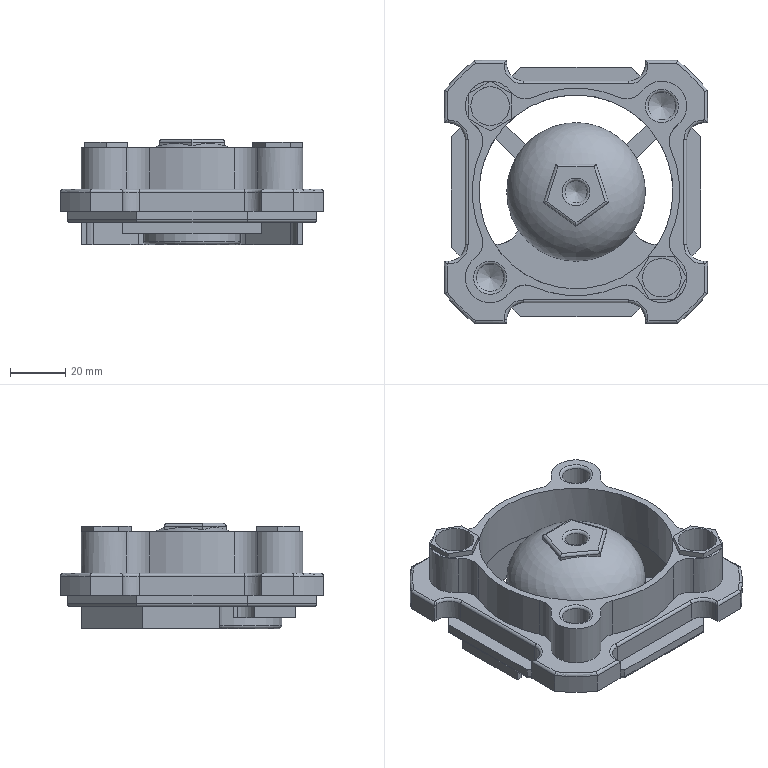NC program | NX | posted with a generic post | part box 95 x 95 x 38 mm
Lines 3621 to 4419 of 59038:
(FIXED_CONTOUR_2 , TOOL : D10R1)
N7186 M6
N7188 G54
N7190 G17 G0 G90 X-4.223 Y-29.7 S3000 M3
N7192 G43 Z10. H0
N7194 Z-8.
N7196 G94 G1 Z-19. F2500.
N7198 Y-29.698 Z-18.791
N7200 X-4.222 Y-29.695 Z-18.644
N7202 Y-29.691 Z-18.511
N7204 X-4.216 Y-29.652 Z-17.848
N7206 X-4.211 Y-29.614 Z-17.452
N7208 X-4.2 Y-29.537 Z-16.864
N7210 X-4.189 Y-29.461 Z-16.413
N7212 X-4.178 Y-29.384 Z-16.03
N7214 X-4.156 Y-29.231 Z-15.382
N7216 X-4.135 Y-29.078 Z-14.842
N7218 X-4.113 Y-28.925 Z-14.361
N7220 X-4.091 Y-28.772 Z-13.934
N7222 X-4.069 Y-28.619 Z-13.541
N7224 X-4.047 Y-28.466 Z-13.176
N7226 X-4.004 Y-28.16 Z-12.513
N7228 X-3.96 Y-27.853 Z-11.919
N7230 X-3.917 Y-27.547 Z-11.378
N7232 X-3.873 Y-27.241 Z-10.881
N7234 X-3.83 Y-26.935 Z-10.417
N7236 X-3.786 Y-26.629 Z-9.983
N7238 X-3.743 Y-26.322 Z-9.575
N7240 X-3.699 Y-26.016 Z-9.189
N7242 X-3.656 Y-25.71 Z-8.821
N7244 X-3.612 Y-25.404 Z-8.473
N7246 X-3.569 Y-25.098 Z-8.141
N7248 X-3.525 Y-24.791 Z-7.823
N7250 X-3.438 Y-24.179 Z-7.226
N7252 X-3.351 Y-23.567 Z-6.674
N7254 X-3.264 Y-22.954 Z-6.162
N7256 X-3.177 Y-22.342 Z-5.685
N7258 X-3.09 Y-21.73 Z-5.239
N7260 X-3.003 Y-21.117 Z-4.823
N7262 X-2.915 Y-20.505 Z-4.432
N7264 X-2.828 Y-19.892 Z-4.065
N7266 X-2.717 Y-19.109 Z-3.628
N7268 X-2.606 Y-18.325 Z-3.224
N7270 X-2.494 Y-17.541 Z-2.851
N7272 X-2.383 Y-16.757 Z-2.506
N7274 X-2.382 Y-16.756 Z-2.
N7276 Y-16.755 Z-1.929
N7278 X-2.381 Y-16.748 Z-1.827
N7280 X-2.38 Y-16.741 Z-1.766
N7282 X-2.378 Y-16.727 Z-1.683
N7284 X-2.374 Y-16.7 Z-1.551
N7286 X-2.367 Y-16.645 Z-1.371
N7288 X-2.359 Y-16.59 Z-1.237
N7290 X-2.351 Y-16.535 Z-1.128
N7292 X-2.335 Y-16.425 Z-0.946
N7294 X-2.32 Y-16.315 Z-0.8
N7296 X-2.304 Y-16.204 Z-0.676
N7298 X-2.288 Y-16.094 Z-0.571
N7300 X-2.257 Y-15.874 Z-0.4
N7302 X-2.226 Y-15.654 Z-0.269
N7304 X-2.194 Y-15.434 Z-0.168
N7306 X-2.163 Y-15.213 Z-0.093
N7308 X-2.132 Y-14.993 Z-0.041
N7310 X-2.11 Y-14.84 Z-0.019
N7312 X-2.088 Y-14.687 Z-0.005
N7314 X-2.045 Y-14.381 Z0.
N7316 X-1.434 Y-10.083
N7318 X-1.371 Y-10.128
N7320 X-1.953 Y-14.422
N7322 X-1.994 Y-14.728 Z-0.004
N7324 X-2.015 Y-14.881 Z-0.017
N7326 X-2.036 Y-15.034 Z-0.038
N7328 X-2.066 Y-15.256 Z-0.089
N7330 X-2.096 Y-15.478 Z-0.164
N7332 X-2.126 Y-15.7 Z-0.265
N7334 X-2.156 Y-15.922 Z-0.396
N7336 X-2.186 Y-16.144 Z-0.566
N7338 X-2.201 Y-16.255 Z-0.672
N7340 X-2.216 Y-16.366 Z-0.795
N7342 X-2.231 Y-16.478 Z-0.942
N7344 X-2.246 Y-16.589 Z-1.124
N7346 X-2.254 Y-16.644 Z-1.234
N7348 X-2.261 Y-16.7 Z-1.368
N7350 X-2.269 Y-16.755 Z-1.548
N7352 X-2.272 Y-16.783 Z-1.681
N7354 X-2.274 Y-16.797 Z-1.763
N7356 X-2.276 Y-16.811 Z-1.922
N7358 Y-16.812 Z-2.
N7360 Y-16.813 Z-2.523
N7362 X-2.382 Y-17.592 Z-2.867
N7364 X-2.487 Y-18.37 Z-3.238
N7366 X-2.593 Y-19.149 Z-3.64
N7368 X-2.698 Y-19.928 Z-4.075
N7370 X-2.781 Y-20.54 Z-4.443
N7372 X-2.864 Y-21.152 Z-4.833
N7374 X-2.947 Y-21.764 Z-5.249
N7376 X-3.03 Y-22.376 Z-5.695
N7378 X-3.112 Y-22.987 Z-6.172
N7380 X-3.195 Y-23.599 Z-6.684
N7382 X-3.278 Y-24.211 Z-7.235
N7384 X-3.361 Y-24.823 Z-7.832
N7386 X-3.402 Y-25.129 Z-8.15
N7388 X-3.444 Y-25.435 Z-8.482
N7390 X-3.485 Y-25.74 Z-8.83
N7392 X-3.527 Y-26.046 Z-9.197
N7394 X-3.568 Y-26.352 Z-9.583
N7396 X-3.609 Y-26.658 Z-9.99
N7398 X-3.651 Y-26.964 Z-10.424
N7400 X-3.692 Y-27.27 Z-10.887
N7402 X-3.734 Y-27.576 Z-11.385
N7404 X-3.775 Y-27.882 Z-11.924
N7406 X-3.816 Y-28.188 Z-12.518
N7408 X-3.858 Y-28.494 Z-13.181
N7410 X-3.879 Y-28.647 Z-13.545
N7412 X-3.899 Y-28.799 Z-13.938
N7414 X-3.92 Y-28.952 Z-14.365
N7416 X-3.941 Y-29.105 Z-14.845
N7418 X-3.961 Y-29.258 Z-15.385
N7420 X-3.982 Y-29.411 Z-16.031
N7422 X-3.992 Y-29.488 Z-16.414
N7424 X-4.003 Y-29.564 Z-16.864
N7426 X-4.013 Y-29.641 Z-17.451
N7428 X-4.018 Y-29.679 Z-17.846
N7430 X-4.024 Y-29.717 Z-18.505
N7432 X-4.025 Y-29.727 Z-19.
N7434 X-3.827 Y-29.754
N7436 X-3.826 Y-29.744 Z-18.499
N7438 X-3.821 Y-29.706 Z-17.845
N7440 X-3.816 Y-29.667 Z-17.45
N7442 X-3.806 Y-29.591 Z-16.865
N7444 X-3.796 Y-29.515 Z-16.415
N7446 X-3.786 Y-29.438 Z-16.033
N7448 X-3.767 Y-29.285 Z-15.387
N7450 X-3.747 Y-29.133 Z-14.848
N7452 X-3.727 Y-28.98 Z-14.369
N7454 X-3.708 Y-28.827 Z-13.942
N7456 X-3.688 Y-28.674 Z-13.549
N7458 X-3.668 Y-28.521 Z-13.185
N7460 X-3.629 Y-28.216 Z-12.524
N7462 X-3.59 Y-27.91 Z-11.93
N7464 X-3.55 Y-27.605 Z-11.391
N7466 X-3.511 Y-27.299 Z-10.894
N7468 X-3.472 Y-26.993 Z-10.431
N7470 X-3.432 Y-26.688 Z-9.998
N7472 X-3.393 Y-26.382 Z-9.591
N7474 X-3.354 Y-26.077 Z-9.205
N7476 X-3.315 Y-25.771 Z-8.839
N7478 X-3.275 Y-25.465 Z-8.49
N7480 X-3.236 Y-25.16 Z-8.159
N7482 X-3.197 Y-24.854 Z-7.841
N7484 X-3.118 Y-24.243 Z-7.245
N7486 X-3.039 Y-23.632 Z-6.694
N7488 X-2.961 Y-23.021 Z-6.182
N7490 X-2.882 Y-22.409 Z-5.705
N7492 X-2.804 Y-21.798 Z-5.26
N7494 X-2.725 Y-21.187 Z-4.844
N7496 X-2.646 Y-20.576 Z-4.453
N7498 X-2.568 Y-19.965 Z-4.086
N7500 X-2.468 Y-19.19 Z-3.653
N7502 X-2.368 Y-18.415 Z-3.252
N7504 X-2.269 Y-17.641 Z-2.882
N7506 X-2.169 Y-16.866 Z-2.539
N7508 Y-16.865 Z-2.
N7510 Y-16.864 Z-1.934
N7512 Y-16.861 Z-1.868
N7514 X-2.168 Y-16.857 Z-1.828
N7516 X-2.167 Y-16.85 Z-1.765
N7518 X-2.165 Y-16.836 Z-1.682
N7520 X-2.162 Y-16.808 Z-1.548
N7522 X-2.155 Y-16.752 Z-1.367
N7524 X-2.147 Y-16.696 Z-1.232
N7526 X-2.14 Y-16.64 Z-1.122
N7528 X-2.126 Y-16.529 Z-0.94
N7530 X-2.111 Y-16.417 Z-0.792
N7532 X-2.097 Y-16.305 Z-0.668
N7534 X-2.083 Y-16.193 Z-0.563
N7536 X-2.054 Y-15.97 Z-0.392
N7538 X-2.025 Y-15.746 Z-0.261
N7540 X-1.996 Y-15.522 Z-0.161
N7542 X-1.968 Y-15.299 Z-0.087
N7544 X-1.939 Y-15.075 Z-0.037
N7546 X-1.919 Y-14.922 Z-0.016
N7548 X-1.9 Y-14.769 Z-0.004
N7550 X-1.86 Y-14.464 Z0.
N7552 X-1.309 Y-10.174
N7554 X-1.245 Y-10.22
N7556 X-1.767 Y-14.505
N7558 X-1.805 Y-14.81 Z-0.004
N7560 X-1.823 Y-14.963 Z-0.015
N7562 X-1.842 Y-15.115 Z-0.035
N7564 X-1.869 Y-15.34 Z-0.085
N7566 X-1.897 Y-15.565 Z-0.158
N7568 X-1.924 Y-15.79 Z-0.259
N7570 X-1.951 Y-16.015 Z-0.389
N7572 X-1.979 Y-16.24 Z-0.56
N7574 X-1.992 Y-16.352 Z-0.665
N7576 X-2.006 Y-16.464 Z-0.789
N7578 X-2.02 Y-16.577 Z-0.937
N7580 X-2.034 Y-16.689 Z-1.119
N7582 X-2.04 Y-16.745 Z-1.23
N7584 X-2.047 Y-16.802 Z-1.365
N7586 X-2.054 Y-16.858 Z-1.545
N7588 X-2.058 Y-16.886 Z-1.678
N7590 X-2.059 Y-16.9 Z-1.761
N7592 X-2.061 Y-16.914 Z-1.918
N7594 Y-16.916 Z-2.
N7596 Z-2.554
N7598 X-2.155 Y-17.687 Z-2.896
N7600 X-2.249 Y-18.458 Z-3.265
N7602 X-2.343 Y-19.229 Z-3.665
N7604 X-2.437 Y-20. Z-4.096
N7606 X-2.511 Y-20.61 Z-4.464
N7608 X-2.586 Y-21.221 Z-4.854
N7610 X-2.66 Y-21.831 Z-5.27
N7612 X-2.734 Y-22.442 Z-5.715
N7614 X-2.809 Y-23.052 Z-6.192
N7616 X-2.883 Y-23.663 Z-6.703
N7618 X-2.958 Y-24.273 Z-7.254
N7620 X-3.032 Y-24.884 Z-7.85
N7622 X-3.069 Y-25.189 Z-8.167
N7624 X-3.106 Y-25.495 Z-8.498
N7626 X-3.144 Y-25.8 Z-8.846
N7628 X-3.181 Y-26.105 Z-9.212
N7630 X-3.218 Y-26.41 Z-9.598
N7632 X-3.255 Y-26.716 Z-10.004
N7634 X-3.292 Y-27.021 Z-10.437
N7636 X-3.33 Y-27.326 Z-10.899
N7638 X-3.367 Y-27.631 Z-11.396
N7640 X-3.404 Y-27.937 Z-11.934
N7642 X-3.441 Y-28.242 Z-12.527
N7644 X-3.478 Y-28.547 Z-13.188
N7646 X-3.497 Y-28.7 Z-13.551
N7648 X-3.516 Y-28.852 Z-13.943
N7650 X-3.534 Y-29.005 Z-14.369
N7652 X-3.553 Y-29.158 Z-14.847
N7654 X-3.571 Y-29.31 Z-15.385
N7656 X-3.59 Y-29.463 Z-16.029
N7658 X-3.599 Y-29.539 Z-16.41
N7660 X-3.609 Y-29.616 Z-16.857
N7662 X-3.618 Y-29.692 Z-17.44
N7664 X-3.623 Y-29.73 Z-17.83
N7666 X-3.627 Y-29.768 Z-18.462
N7668 X-3.628 Y-29.778 Z-19.
N7670 X-3.43 Y-29.802
N7672 X-3.429 Y-29.792 Z-18.504
N7674 X-3.424 Y-29.754 Z-17.848
N7676 X-3.42 Y-29.716 Z-17.455
N7678 X-3.411 Y-29.639 Z-16.87
N7680 X-3.402 Y-29.563 Z-16.421
N7682 X-3.394 Y-29.487 Z-16.039
N7684 X-3.376 Y-29.335 Z-15.394
N7686 X-3.359 Y-29.182 Z-14.856
N7688 X-3.341 Y-29.03 Z-14.378
N7690 X-3.324 Y-28.877 Z-13.951
N7692 X-3.306 Y-28.725 Z-13.56
N7694 X-3.288 Y-28.572 Z-13.196
N7696 X-3.253 Y-28.267 Z-12.536
N7698 X-3.218 Y-27.962 Z-11.943
N7700 X-3.183 Y-27.658 Z-11.406
N7702 X-3.148 Y-27.353 Z-10.909
N7704 X-3.113 Y-27.048 Z-10.447
N7706 X-3.078 Y-26.743 Z-10.014
N7708 X-3.043 Y-26.438 Z-9.608
N7710 X-3.008 Y-26.133 Z-9.223
N7712 X-2.973 Y-25.828 Z-8.857
N7714 X-2.937 Y-25.523 Z-8.509
N7716 X-2.902 Y-25.218 Z-8.177
N7718 X-2.867 Y-24.913 Z-7.86
N7720 X-2.797 Y-24.303 Z-7.265
N7722 X-2.727 Y-23.694 Z-6.714
N7724 X-2.657 Y-23.084 Z-6.203
N7726 X-2.587 Y-22.474 Z-5.727
N7728 X-2.516 Y-21.864 Z-5.282
N7730 X-2.446 Y-21.254 Z-4.866
N7732 X-2.376 Y-20.645 Z-4.475
N7734 X-2.306 Y-20.035 Z-4.108
N7736 X-2.217 Y-19.267 Z-3.677
N7738 X-2.129 Y-18.499 Z-3.279
N7740 X-2.041 Y-17.732 Z-2.91
N7742 X-1.952 Y-16.964 Z-2.57
N7744 Y-16.963 Z-2.
N7746 Y-16.962 Z-1.933
N7748 X-1.951 Y-16.948 Z-1.763
N7750 X-1.949 Y-16.934 Z-1.68
N7752 X-1.946 Y-16.906 Z-1.546
N7754 X-1.939 Y-16.849 Z-1.365
N7756 X-1.933 Y-16.793 Z-1.229
N7758 X-1.926 Y-16.736 Z-1.119
N7760 X-1.913 Y-16.624 Z-0.936
N7762 X-1.9 Y-16.511 Z-0.788
N7764 X-1.887 Y-16.398 Z-0.664
N7766 X-1.874 Y-16.285 Z-0.558
N7768 X-1.848 Y-16.059 Z-0.387
N7770 X-1.822 Y-15.833 Z-0.257
N7772 X-1.796 Y-15.608 Z-0.157
N7774 X-1.77 Y-15.382 Z-0.084
N7776 X-1.744 Y-15.156 Z-0.034
N7778 X-1.727 Y-15.004 Z-0.014
N7780 X-1.709 Y-14.851 Z-0.003
N7782 X-1.674 Y-14.546 Z0.
N7784 X-1.182 Y-10.266
N7786 X-1.117 Y-10.313
N7788 X-1.581 Y-14.588
N7790 X-1.613 Y-14.892 Z-0.003
N7792 X-1.63 Y-15.044 Z-0.014
N7794 X-1.646 Y-15.197 Z-0.034
N7796 X-1.671 Y-15.423 Z-0.083
N7798 X-1.696 Y-15.649 Z-0.156
N7800 X-1.72 Y-15.876 Z-0.256
N7802 X-1.745 Y-16.102 Z-0.386
N7804 X-1.769 Y-16.328 Z-0.557
N7806 X-1.781 Y-16.441 Z-0.662
N7808 X-1.789 Y-16.512 Z-0.738
N7810 X-1.794 Y-16.554 Z-0.787
N7812 X-1.806 Y-16.668 Z-0.934
N7814 X-1.818 Y-16.781 Z-1.117
N7816 X-1.824 Y-16.837 Z-1.228
N7818 X-1.83 Y-16.894 Z-1.363
N7820 X-1.836 Y-16.95 Z-1.545
N7822 X-1.84 Y-16.979 Z-1.679
N7824 X-1.841 Y-16.993 Z-1.762
N7826 X-1.843 Y-17.007 Z-1.927
N7828 Y-17.009 Z-2.
N7830 Z-2.584
N7832 X-1.926 Y-17.774 Z-2.924
N7834 X-2.009 Y-18.539 Z-3.292
N7836 X-2.092 Y-19.304 Z-3.689
N7838 X-2.174 Y-20.069 Z-4.119
N7840 X-2.24 Y-20.678 Z-4.487
N7842 X-2.306 Y-21.287 Z-4.877
N7844 X-2.372 Y-21.896 Z-5.293
N7846 X-2.438 Y-22.505 Z-5.738
N7848 X-2.504 Y-23.114 Z-6.214
N7850 X-2.57 Y-23.723 Z-6.725
N7852 X-2.636 Y-24.332 Z-7.275
N7854 X-2.702 Y-24.942 Z-7.87
N7856 X-2.735 Y-25.246 Z-8.187
N7858 X-2.768 Y-25.551 Z-8.518
N7860 X-2.801 Y-25.855 Z-8.866
N7862 X-2.834 Y-26.16 Z-9.232
N7864 X-2.867 Y-26.464 Z-9.617
N7866 X-2.9 Y-26.769 Z-10.022
N7868 X-2.933 Y-27.073 Z-10.455
N7870 X-2.966 Y-27.378 Z-10.917
N7872 X-2.999 Y-27.682 Z-11.413
N7874 X-3.032 Y-27.987 Z-11.95
N7876 X-3.065 Y-28.291 Z-12.542
N7878 X-3.098 Y-28.596 Z-13.202
N7880 X-3.115 Y-28.748 Z-13.565
N7882 X-3.131 Y-28.9 Z-13.956
N7884 X-3.148 Y-29.053 Z-14.383
N7886 X-3.164 Y-29.205 Z-14.86
N7888 X-3.181 Y-29.357 Z-15.398
N7890 X-3.197 Y-29.509 Z-16.042
N7892 X-3.205 Y-29.586 Z-16.423
N7894 X-3.214 Y-29.662 Z-16.872
N7896 X-3.222 Y-29.738 Z-17.456
N7898 X-3.226 Y-29.776 Z-17.849
N7900 X-3.23 Y-29.814 Z-18.504
N7902 X-3.231 Y-29.824 Z-19.
N7904 X-3.032 Y-29.844
N7906 X-3.031 Y-29.835 Z-18.467
N7908 X-3.028 Y-29.796 Z-17.834
N7910 X-3.024 Y-29.758 Z-17.445
N7912 X-3.016 Y-29.682 Z-16.864
N7914 X-3.008 Y-29.606 Z-16.418
N7916 X-3.001 Y-29.53 Z-16.038
N7918 X-2.985 Y-29.378 Z-15.396
N7920 X-2.97 Y-29.226 Z-14.86
N7922 X-2.954 Y-29.074 Z-14.383
N7924 X-2.939 Y-28.922 Z-13.957
N7926 X-2.923 Y-28.77 Z-13.567
N7928 X-2.908 Y-28.618 Z-13.205
N7930 X-2.877 Y-28.314 Z-12.546
N7932 X-2.846 Y-28.01 Z-11.954
N7934 X-2.815 Y-27.706 Z-11.418
N7936 X-2.784 Y-27.402 Z-10.922
N7938 X-2.753 Y-27.097 Z-10.462
N7940 X-2.722 Y-26.793 Z-10.029
N7942 X-2.692 Y-26.489 Z-9.624
N7944 X-2.661 Y-26.185 Z-9.24
N7946 X-2.63 Y-25.881 Z-8.875
N7948 X-2.599 Y-25.577 Z-8.527
N7950 X-2.568 Y-25.273 Z-8.196
N7952 X-2.537 Y-24.969 Z-7.879
N7954 X-2.475 Y-24.36 Z-7.284
N7956 X-2.413 Y-23.752 Z-6.735
N7958 X-2.352 Y-23.144 Z-6.224
N7960 X-2.29 Y-22.536 Z-5.748
N7962 X-2.228 Y-21.928 Z-5.304
N7964 X-2.166 Y-21.319 Z-4.888
N7966 X-2.104 Y-20.711 Z-4.498
N7968 X-2.043 Y-20.103 Z-4.13
N7970 X-1.965 Y-19.34 Z-3.701
N7972 X-1.888 Y-18.577 Z-3.304
N7974 X-1.81 Y-17.814 Z-2.937
N7976 X-1.733 Y-17.051 Z-2.596
N7978 X-1.732 Y-17.05 Z-2.
N7980 Y-17.049 Z-1.924
N7982 Y-17.046 Z-1.864
N7984 Y-17.042 Z-1.824
N7986 X-1.731 Y-17.035 Z-1.761
N7988 X-1.729 Y-17.021 Z-1.679
N7990 X-1.727 Y-16.993 Z-1.544
N7992 X-1.721 Y-16.936 Z-1.363
N7994 X-1.715 Y-16.879 Z-1.228
N7996 X-1.709 Y-16.823 Z-1.117
N7998 X-1.698 Y-16.709 Z-0.934
N8000 X-1.686 Y-16.593 Z-0.782
N8002 X-1.681 Y-16.54 Z-0.722
N8004 X-1.675 Y-16.483 Z-0.662
N8006 X-1.663 Y-16.37 Z-0.557
N8008 X-1.64 Y-16.143 Z-0.386
N8010 X-1.617 Y-15.917 Z-0.256
N8012 X-1.594 Y-15.69 Z-0.156
N8014 X-1.571 Y-15.464 Z-0.083
N8016 X-1.548 Y-15.237 Z-0.034
N8018 X-1.533 Y-15.085 Z-0.014
N8020 X-1.517 Y-14.933 Z-0.003
N8022 X-1.486 Y-14.629 Z0.
N8024 X-1.053 Y-10.36
N8026 X-0.987 Y-10.407
N8028 X-1.392 Y-14.67
N8030 X-1.421 Y-14.974 Z-0.003
N8032 X-1.435 Y-15.126 Z-0.014
N8034 X-1.45 Y-15.278 Z-0.034
N8036 X-1.471 Y-15.504 Z-0.083
N8038 X-1.493 Y-15.73 Z-0.157
N8040 X-1.514 Y-15.957 Z-0.257
N8042 X-1.535 Y-16.183 Z-0.387
N8044 X-1.557 Y-16.41 Z-0.558
N8046 X-1.568 Y-16.523 Z-0.663
N8048 X-1.574 Y-16.594 Z-0.739
N8050 X-1.578 Y-16.636 Z-0.787
N8052 X-1.589 Y-16.749 Z-0.935
N8054 X-1.6 Y-16.862 Z-1.118
N8056 X-1.611 Y-16.976 Z-1.364
N8058 X-1.616 Y-17.032 Z-1.545
N8060 X-1.619 Y-17.064 Z-1.7
N8062 X-1.62 Y-17.075 Z-1.763
N8064 X-1.621 Y-17.089 Z-1.932
N8066 X-1.622 Y-17.091 Z-2.
N8068 Z-2.609
N8070 X-1.694 Y-17.852 Z-2.949
N8072 X-1.766 Y-18.614 Z-3.317
N8074 X-1.838 Y-19.375 Z-3.714
N8076 X-1.911 Y-20.137 Z-4.143
N8078 X-1.968 Y-20.744 Z-4.509
N8080 X-2.026 Y-21.351 Z-4.9
N8082 X-2.083 Y-21.959 Z-5.316
N8084 X-2.141 Y-22.566 Z-5.759
N8086 X-2.199 Y-23.173 Z-6.235
N8088 X-2.256 Y-23.781 Z-6.746
N8090 X-2.314 Y-24.388 Z-7.295
N8092 X-2.372 Y-24.995 Z-7.89
N8094 X-2.4 Y-25.299 Z-8.206
N8096 X-2.429 Y-25.603 Z-8.537
N8098 X-2.458 Y-25.906 Z-8.885
N8100 X-2.487 Y-26.21 Z-9.249
N8102 X-2.516 Y-26.514 Z-9.633
N8104 X-2.544 Y-26.818 Z-10.038
N8106 X-2.573 Y-27.121 Z-10.471
N8108 X-2.602 Y-27.425 Z-10.931
N8110 X-2.631 Y-27.729 Z-11.426
N8112 X-2.66 Y-28.032 Z-11.962
N8114 X-2.689 Y-28.336 Z-12.553
N8116 X-2.717 Y-28.64 Z-13.211
N8118 X-2.732 Y-28.791 Z-13.574
N8120 X-2.746 Y-28.943 Z-13.964
N8122 X-2.761 Y-29.095 Z-14.389
N8124 X-2.775 Y-29.247 Z-14.865
N8126 X-2.789 Y-29.399 Z-15.401
N8128 X-2.804 Y-29.551 Z-16.043
N8130 X-2.811 Y-29.627 Z-16.423
N8132 X-2.818 Y-29.702 Z-16.869
N8134 X-2.825 Y-29.778 Z-17.45
N8136 X-2.829 Y-29.816 Z-17.84
N8138 X-2.833 Y-29.854 Z-18.478
N8140 X-2.834 Y-29.864 Z-19.
N8142 X-2.634 Y-29.882
N8144 Y-29.872 Z-18.497
N8146 X-2.63 Y-29.834 Z-17.849
N8148 X-2.627 Y-29.796 Z-17.458
N8150 X-2.62 Y-29.721 Z-16.877
N8152 X-2.614 Y-29.645 Z-16.429
N8154 X-2.607 Y-29.569 Z-16.049
N8156 X-2.594 Y-29.417 Z-15.407
N8158 X-2.58 Y-29.266 Z-14.872
N8160 X-2.567 Y-29.114 Z-14.396
N8162 X-2.553 Y-28.963 Z-13.97
N8164 X-2.54 Y-28.811 Z-13.581
N8166 X-2.527 Y-28.659 Z-13.219
N8168 X-2.5 Y-28.356 Z-12.561
N8170 X-2.473 Y-28.053 Z-11.97
N8172 X-2.446 Y-27.75 Z-11.435
N8174 X-2.42 Y-27.447 Z-10.94
N8176 X-2.393 Y-27.143 Z-10.48
N8178 X-2.366 Y-26.84 Z-10.048
N8180 X-2.34 Y-26.537 Z-9.643
N8182 X-2.313 Y-26.234 Z-9.26
N8184 X-2.286 Y-25.93 Z-8.895
N8186 X-2.259 Y-25.627 Z-8.548
N8188 X-2.233 Y-25.324 Z-8.217
N8190 X-2.206 Y-25.021 Z-7.901
N8192 X-2.152 Y-24.414 Z-7.307
N8194 X-2.099 Y-23.808 Z-6.757
N8196 X-2.046 Y-23.202 Z-6.247
N8198 X-1.992 Y-22.595 Z-5.772
N8200 X-1.939 Y-21.989 Z-5.328
N8202 X-1.885 Y-21.382 Z-4.913
N8204 X-1.832 Y-20.776 Z-4.522
N8206 X-1.778 Y-20.169 Z-4.155
N8208 X-1.711 Y-19.409 Z-3.726
N8210 X-1.644 Y-18.649 Z-3.329
N8212 X-1.577 Y-17.888 Z-2.961
N8214 X-1.51 Y-17.128 Z-2.621
N8216 Y-17.127 Z-2.
N8218 Y-17.126 Z-1.937
N8220 Y-17.122 Z-1.868
N8222 X-1.509 Y-17.112 Z-1.764
N8224 X-1.507 Y-17.098 Z-1.681
N8226 X-1.505 Y-17.069 Z-1.546
N8228 X-1.5 Y-17.013 Z-1.365
N8230 X-1.49 Y-16.9 Z-1.119
N8232 X-1.48 Y-16.787 Z-0.936
N8234 X-1.47 Y-16.674 Z-0.788
N8236 X-1.46 Y-16.561 Z-0.664
N8238 X-1.45 Y-16.448 Z-0.559
N8240 X-1.43 Y-16.222 Z-0.388
N8242 X-1.41 Y-15.996 Z-0.258
N8244 X-1.39 Y-15.77 Z-0.158
N8246 X-1.37 Y-15.544 Z-0.085
N8248 X-1.35 Y-15.318 Z-0.035
N8250 X-1.337 Y-15.166 Z-0.015
N8252 X-1.324 Y-15.015 Z-0.004
N8254 X-1.297 Y-14.712 Z0.
N8256 X-0.922 Y-10.455
N8258 X-0.855 Y-10.503
N8260 X-1.202 Y-14.753
N8262 X-1.226 Y-15.056 Z-0.004
N8264 X-1.251 Y-15.359 Z-0.036
N8266 X-1.269 Y-15.584 Z-0.087
N8268 X-1.288 Y-15.809 Z-0.161
N8270 X-1.306 Y-16.034 Z-0.26
N8272 X-1.324 Y-16.259 Z-0.39
N8274 X-1.343 Y-16.484 Z-0.562
N8276 X-1.352 Y-16.597 Z-0.666
N8278 X-1.361 Y-16.709 Z-0.79
N8280 X-1.37 Y-16.822 Z-0.937
N8282 X-1.379 Y-16.934 Z-1.119
N8284 X-1.388 Y-17.047 Z-1.365
N8286 X-1.393 Y-17.103 Z-1.545
N8288 X-1.395 Y-17.131 Z-1.679
N8290 X-1.398 Y-17.159 Z-1.92
N8292 Y-17.161 Z-2.
N8294 Z-2.631
N8296 X-1.46 Y-17.922 Z-2.972
N8298 X-1.522 Y-18.682 Z-3.34
N8300 X-1.584 Y-19.442 Z-3.738
N8302 X-1.646 Y-20.202 Z-4.168
N8304 X-1.695 Y-20.808 Z-4.534
N8306 X-1.744 Y-21.413 Z-4.925
N8308 X-1.793 Y-22.019 Z-5.341
N8310 X-1.843 Y-22.624 Z-5.784
N8312 X-1.892 Y-23.23 Z-6.259
N8314 X-1.941 Y-23.835 Z-6.769
N8316 X-1.991 Y-24.441 Z-7.318
N8318 X-2.04 Y-25.046 Z-7.912
N8320 X-2.065 Y-25.349 Z-8.228
N8322 X-2.089 Y-25.652 Z-8.559
N8324 X-2.114 Y-25.954 Z-8.906
N8326 X-2.139 Y-26.257 Z-9.27
N8328 X-2.163 Y-26.56 Z-9.653
N8330 X-2.188 Y-26.863 Z-10.058
N8332 X-2.213 Y-27.165 Z-10.49
N8334 X-2.237 Y-27.468 Z-10.949
N8336 X-2.262 Y-27.771 Z-11.444
N8338 X-2.287 Y-28.074 Z-11.978
N8340 X-2.311 Y-28.376 Z-12.569
N8342 X-2.336 Y-28.679 Z-13.226
N8344 X-2.348 Y-28.83 Z-13.588
N8346 X-2.361 Y-28.982 Z-13.977
N8348 X-2.373 Y-29.133 Z-14.403
N8350 X-2.385 Y-29.284 Z-14.878
N8352 X-2.398 Y-29.436 Z-15.413
N8354 X-2.41 Y-29.587 Z-16.055
N8356 X-2.416 Y-29.663 Z-16.434
N8358 X-2.422 Y-29.739 Z-16.883
N8360 X-2.428 Y-29.814 Z-17.464
N8362 X-2.432 Y-29.852 Z-17.856
N8364 X-2.435 Y-29.89 Z-18.512
N8366 Y-29.9 Z-19.
N8368 X-2.236 Y-29.915
N8370 X-2.235 Y-29.905 Z-18.454
N8372 X-2.232 Y-29.867 Z-17.832
N8374 X-2.23 Y-29.829 Z-17.446
N8376 X-2.224 Y-29.754 Z-16.87
N8378 X-2.218 Y-29.678 Z-16.426
N8380 X-2.213 Y-29.603 Z-16.048
N8382 X-2.201 Y-29.451 Z-15.408
N8384 X-2.19 Y-29.3 Z-14.876
N8386 X-2.179 Y-29.149 Z-14.402
N8388 X-2.168 Y-28.998 Z-13.977
N8390 X-2.156 Y-28.847 Z-13.588
N8392 X-2.145 Y-28.696 Z-13.227
N8394 X-2.122 Y-28.394 Z-12.571
N8396 X-2.1 Y-28.091 Z-11.982
N8398 X-2.077 Y-27.789 Z-11.449
N8400 X-2.055 Y-27.487 Z-10.954
N8402 X-2.032 Y-27.185 Z-10.496
N8404 X-2.009 Y-26.883 Z-10.065
N8406 X-1.987 Y-26.58 Z-9.66
N8408 X-1.964 Y-26.278 Z-9.278
N8410 X-1.942 Y-25.976 Z-8.914
N8412 X-1.919 Y-25.674 Z-8.568
N8414 X-1.896 Y-25.372 Z-8.237
N8416 X-1.874 Y-25.069 Z-7.921
N8418 X-1.829 Y-24.465 Z-7.328
N8420 X-1.784 Y-23.861 Z-6.779
N8422 X-1.738 Y-23.256 Z-6.27
N8424 X-1.693 Y-22.652 Z-5.795
N8426 X-1.648 Y-22.047 Z-5.352
N8428 X-1.603 Y-21.443 Z-4.937
N8430 X-1.558 Y-20.838 Z-4.546
N8432 X-1.512 Y-20.234 Z-4.18
N8434 X-1.456 Y-19.474 Z-3.75
N8436 X-1.399 Y-18.714 Z-3.351
N8438 X-1.342 Y-17.953 Z-2.982
N8440 X-1.285 Y-17.193 Z-2.64
N8442 Y-17.192 Z-2.
N8444 Y-17.191 Z-1.93
N8446 X-1.284 Y-17.177 Z-1.763
N8448 X-1.283 Y-17.163 Z-1.682
N8450 X-1.281 Y-17.135 Z-1.547
N8452 X-1.277 Y-17.079 Z-1.367
N8454 X-1.268 Y-16.967 Z-1.122
N8456 X-1.26 Y-16.855 Z-0.94
N8458 X-1.252 Y-16.743 Z-0.792
N8460 X-1.243 Y-16.631 Z-0.669
N8462 X-1.237 Y-16.547 Z-0.591
N8464 X-1.235 Y-16.519 Z-0.565
N8466 X-1.218 Y-16.295 Z-0.393
N8468 X-1.201 Y-16.071 Z-0.263
N8470 X-1.185 Y-15.847 Z-0.163
N8472 X-1.168 Y-15.623 Z-0.089
N8474 X-1.151 Y-15.399 Z-0.038
N8476 X-1.128 Y-15.096 Z-0.004
N8478 X-1.106 Y-14.794 Z0.
N8480 X-0.789 Y-10.552
N8482 X-0.721 Y-10.601
N8484 X-1.01 Y-14.836
N8486 X-1.03 Y-15.137 Z-0.005
N8488 X-1.051 Y-15.439 Z-0.041
N8490 X-1.066 Y-15.662 Z-0.093
N8492 X-1.081 Y-15.884 Z-0.167
N8494 X-1.096 Y-16.107 Z-0.267
N8496 X-1.111 Y-16.329 Z-0.397
N8498 X-1.126 Y-16.552 Z-0.569
N8500 X-1.134 Y-16.663 Z-0.673
N8502 X-1.142 Y-16.774 Z-0.796
N8504 X-1.146 Y-16.84 Z-0.88
N8506 X-1.149 Y-16.886 Z-0.942
N8508 X-1.157 Y-16.997 Z-1.124
N8510 X-1.164 Y-17.108 Z-1.368
N8512 X-1.168 Y-17.164 Z-1.547
N8514 X-1.17 Y-17.192 Z-1.681
N8516 X-1.172 Y-17.219 Z-1.921
N8518 Y-17.221 Z-2.
N8520 Z-2.649
N8522 X-1.224 Y-17.983 Z-2.992
N8524 X-1.276 Y-18.744 Z-3.362
N8526 X-1.327 Y-19.505 Z-3.762
N8528 X-1.379 Y-20.266 Z-4.193
N8530 X-1.42 Y-20.869 Z-4.559
N8532 X-1.461 Y-21.473 Z-4.95
N8534 X-1.502 Y-22.076 Z-5.366
N8536 X-1.543 Y-22.679 Z-5.809
N8538 X-1.584 Y-23.283 Z-6.283
N8540 X-1.625 Y-23.886 Z-6.792
N8542 X-1.667 Y-24.489 Z-7.341
N8544 X-1.708 Y-25.093 Z-7.933
N8546 X-1.728 Y-25.394 Z-8.25
N8548 X-1.749 Y-25.696 Z-8.58
N8550 X-1.769 Y-25.998 Z-8.926
N8552 X-1.79 Y-26.299 Z-9.29
N8554 X-1.81 Y-26.601 Z-9.672
N8556 X-1.831 Y-26.903 Z-10.076
N8558 X-1.851 Y-27.204 Z-10.507
N8560 X-1.872 Y-27.506 Z-10.965
N8562 X-1.892 Y-27.808 Z-11.46
N8564 X-1.913 Y-28.109 Z-11.993
N8566 X-1.933 Y-28.411 Z-12.581
N8568 X-1.954 Y-28.713 Z-13.237
N8570 X-1.964 Y-28.864 Z-13.598
N8572 X-1.974 Y-29.014 Z-13.986
N8574 X-1.985 Y-29.165 Z-14.412
N8576 X-1.995 Y-29.316 Z-14.886
N8578 X-2.005 Y-29.467 Z-15.419
N8580 X-2.016 Y-29.618 Z-16.059
N8582 X-2.021 Y-29.693 Z-16.437
N8584 X-2.026 Y-29.769 Z-16.884
N8586 X-2.031 Y-29.844 Z-17.462
N8588 X-2.033 Y-29.882 Z-17.852
N8590 X-2.036 Y-29.92 Z-18.498
N8592 X-2.037 Y-29.929 Z-19.
N8594 X-1.837 Y-29.942
N8596 Y-29.932 Z-18.506
N8598 X-1.834 Y-29.894 Z-17.857
N8600 X-1.832 Y-29.857 Z-17.467
N8602 X-1.827 Y-29.782 Z-16.889
N8604 X-1.823 Y-29.706 Z-16.441
N8606 X-1.818 Y-29.631 Z-16.063
N8608 X-1.809 Y-29.48 Z-15.424
N8610 X-1.8 Y-29.33 Z-14.891
N8612 X-1.79 Y-29.179 Z-14.418
N8614 X-1.781 Y-29.029 Z-13.993
N8616 X-1.772 Y-28.878 Z-13.605
N8618 X-1.763 Y-28.728 Z-13.244
N8620 X-1.744 Y-28.427 Z-12.589
N8622 X-1.726 Y-28.125 Z-12.001
N8624 X-1.707 Y-27.824 Z-11.468
N8626 X-1.689 Y-27.523 Z-10.974
N8628 X-1.67 Y-27.222 Z-10.517
N8630 X-1.652 Y-26.921 Z-10.087
N8632 X-1.633 Y-26.62 Z-9.682
N8634 X-1.615 Y-26.319 Z-9.3
N8636 X-1.596 Y-26.018 Z-8.938
N8638 X-1.578 Y-25.717 Z-8.592
N8640 X-1.56 Y-25.416 Z-8.261
N8642 X-1.541 Y-25.114 Z-7.945
N8644 X-1.504 Y-24.512 Z-7.352
N8646 X-1.467 Y-23.91 Z-6.805
N8648 X-1.43 Y-23.308 Z-6.296
N8650 X-1.393 Y-22.706 Z-5.822
N8652 X-1.356 Y-22.103 Z-5.379
N8654 X-1.319 Y-21.501 Z-4.963
N8656 X-1.282 Y-20.899 Z-4.573
N8658 X-1.245 Y-20.297 Z-4.207
N8660 X-1.199 Y-19.535 Z-3.774
N8662 X-1.152 Y-18.772 Z-3.373
N8664 X-1.105 Y-18.01 Z-3.001
N8666 X-1.058 Y-17.248 Z-2.657
N8668 Y-17.247 Z-2.
N8670 Y-17.246 Z-1.927
N8672 X-1.057 Y-17.218 Z-1.683
N8674 X-1.055 Y-17.19 Z-1.549
N8676 X-1.051 Y-17.135 Z-1.371
N8678 X-1.045 Y-17.025 Z-1.127
N8680 X-1.038 Y-16.914 Z-0.946
N8682 X-1.031 Y-16.804 Z-0.8
N8684 X-1.024 Y-16.694 Z-0.678
N8686 X-1.021 Y-16.638 Z-0.624
N8688 X-1.018 Y-16.583 Z-0.574
N8690 X-1.004 Y-16.362 Z-0.402
N8692 X-0.99 Y-16.142 Z-0.272
N8694 X-0.977 Y-15.921 Z-0.172
N8696 X-0.963 Y-15.7 Z-0.097
N8698 X-0.95 Y-15.479 Z-0.044
N8700 X-0.931 Y-15.178 Z-0.006
N8702 X-0.913 Y-14.877 Z0.
N8704 X-0.653 Y-10.65
N8706 X-0.585 Y-10.7
N8708 X-0.816 Y-14.919
N8710 X-0.832 Y-15.219 Z-0.007
N8712 X-0.849 Y-15.52 Z-0.048
N8714 X-0.86 Y-15.738 Z-0.101
N8716 X-0.872 Y-15.957 Z-0.177
N8718 X-0.884 Y-16.176 Z-0.277
N8720 X-0.896 Y-16.394 Z-0.408
N8722 X-0.908 Y-16.613 Z-0.581
N8724 X-0.914 Y-16.722 Z-0.684
N8726 X-0.92 Y-16.832 Z-0.805
N8728 X-0.926 Y-16.941 Z-0.951
N8730 X-0.932 Y-17.05 Z-1.131
N8732 X-0.938 Y-17.16 Z-1.375
N8734 X-0.941 Y-17.214 Z-1.552
N8736 X-0.943 Y-17.242 Z-1.686
N8738 Y-17.255 Z-1.766
N8740 X-0.944 Y-17.269 Z-1.931
N8742 Y-17.271 Z-2.
N8744 Z-2.665
N8746 X-0.986 Y-18.035 Z-3.01
N8748 X-1.028 Y-18.799 Z-3.383
N8750 X-1.07 Y-19.564 Z-3.785
N8752 X-1.111 Y-20.328 Z-4.22
N8754 X-1.144 Y-20.929 Z-4.586
N8756 X-1.177 Y-21.53 Z-4.976
N8758 X-1.21 Y-22.131 Z-5.392
N8760 X-1.243 Y-22.732 Z-5.835
N8762 X-1.276 Y-23.333 Z-6.309
N8764 X-1.309 Y-23.934 Z-6.817
N8766 X-1.341 Y-24.535 Z-7.364
N8768 X-1.374 Y-25.136 Z-7.957
N8770 X-1.391 Y-25.437 Z-8.273
N8772 X-1.407 Y-25.737 Z-8.603
N8774 X-1.424 Y-26.038 Z-8.948
N8776 X-1.44 Y-26.338 Z-9.311